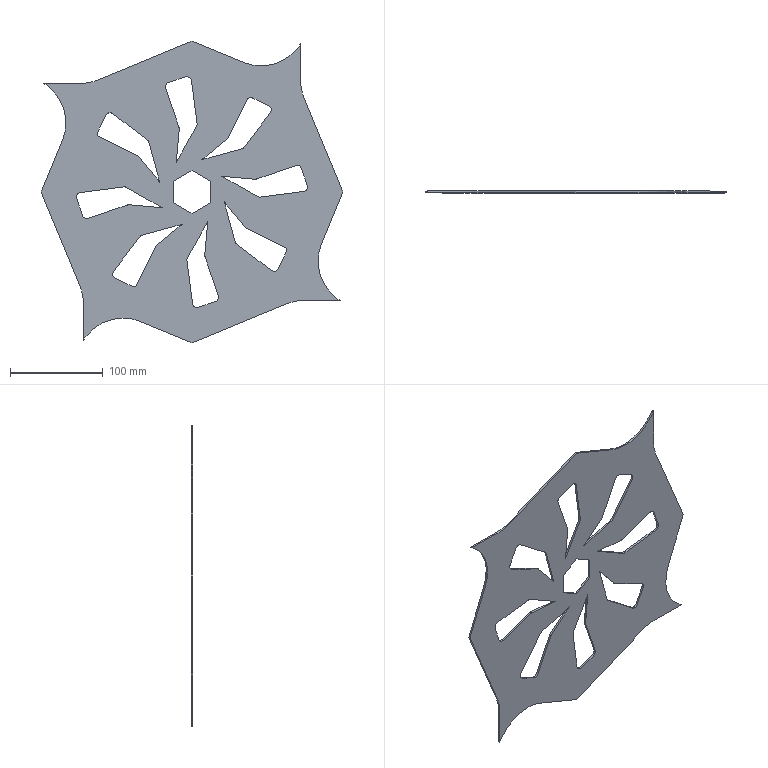Part | SolidWorks | features ICE 3, Extrusion 1, Fillet 1 | 1 solid | 112 faces | box 324.718 x 2 x 324.718 mm | volume 127510 mm3 | plane 64 | cylinder 48 | commonest cylinder face diameters 10 x38 100 x10